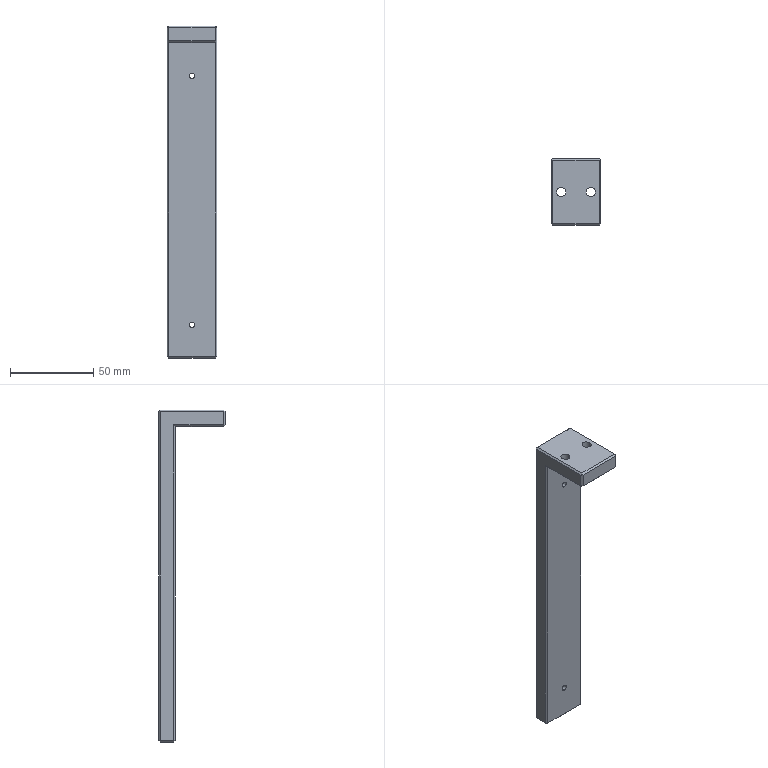Part | SolidWorks | features Chamfer 2, HoleWzd 2, Extrusion 1, ICE 1 | 1 solid | 47 faces | box 30 x 40 x 200 mm | volume 67180 mm3 | plane 35 | cylinder 12 | commonest cylinder face diameters 3.3 x4 5.5 x4 10 x4
STEP:
#1=CARTESIAN_POINT('',(15.,-5.,68.35));
#2=VERTEX_POINT('',#1);
#3=CARTESIAN_POINT('',(15.,-5.,71.65));
#4=VERTEX_POINT('',#3);
#5=CARTESIAN_POINT('',(15.,-5.,70.));
#6=DIRECTION('',(0.,1.,0.));
#7=DIRECTION('',(0.,0.,1.));
#8=AXIS2_PLACEMENT_3D('',#5,#6,#7);
#9=CIRCLE('',#8,1.65);
#10=EDGE_CURVE('',#2,#4,#9,.T.);
#11=ORIENTED_EDGE('',*,*,#10,.F.);
#12=CARTESIAN_POINT('',(15.,5.,68.35));
#13=VERTEX_POINT('',#12);
#14=CARTESIAN_POINT('',(15.,5.,68.35));
#15=DIRECTION('',(0.,1.,0.));
#16=VECTOR('',#15,1000.);
#17=LINE('',#14,#16);
#18=EDGE_CURVE('',#2,#13,#17,.T.);
#19=ORIENTED_EDGE('',*,*,#18,.T.);
#20=CARTESIAN_POINT('',(15.,5.,71.65));
#21=VERTEX_POINT('',#20);
#22=CARTESIAN_POINT('',(15.,5.,70.));
#23=DIRECTION('',(0.,1.,0.));
#24=DIRECTION('',(0.,0.,1.));
#25=AXIS2_PLACEMENT_3D('',#22,#23,#24);
#26=CIRCLE('',#25,1.65);
#27=EDGE_CURVE('',#13,#21,#26,.T.);
#28=ORIENTED_EDGE('',*,*,#27,.T.);
#29=CARTESIAN_POINT('',(15.,5.,71.65));
#30=DIRECTION('',(0.,1.,0.));
#31=VECTOR('',#30,1000.);
#32=LINE('',#29,#31);
#33=EDGE_CURVE('',#4,#21,#32,.T.);
#34=ORIENTED_EDGE('',*,*,#33,.F.);
#35=EDGE_LOOP('',(#11,#19,#28,#34));
#36=FACE_OUTER_BOUND('',#35,.T.);
#37=CARTESIAN_POINT('',(15.,5.,70.));
#38=DIRECTION('',(0.,1.,0.));
#39=DIRECTION('',(0.,0.,1.));
#40=AXIS2_PLACEMENT_3D('',#37,#38,#39);
#41=CYLINDRICAL_SURFACE('',#40,1.65);
#42=ADVANCED_FACE('',(#36),#41,.F.);
#43=CARTESIAN_POINT('',(15.,-5.,-81.65));
#44=VERTEX_POINT('',#43);
#45=CARTESIAN_POINT('',(15.,-5.,-78.35));
#46=VERTEX_POINT('',#45);
#47=CARTESIAN_POINT('',(15.,-5.,-80.));
#48=DIRECTION('',(0.,1.,0.));
#49=DIRECTION('',(0.,0.,1.));
#50=AXIS2_PLACEMENT_3D('',#47,#48,#49);
#51=CIRCLE('',#50,1.65);
#52=EDGE_CURVE('',#44,#46,#51,.T.);
#53=ORIENTED_EDGE('',*,*,#52,.F.);
#54=CARTESIAN_POINT('',(15.,5.,-81.65));
#55=VERTEX_POINT('',#54);
#56=CARTESIAN_POINT('',(15.,5.,-81.65));
#57=DIRECTION('',(0.,1.,0.));
#58=VECTOR('',#57,1000.);
#59=LINE('',#56,#58);
#60=EDGE_CURVE('',#44,#55,#59,.T.);
#61=ORIENTED_EDGE('',*,*,#60,.T.);
#62=CARTESIAN_POINT('',(15.,5.,-78.35));
#63=VERTEX_POINT('',#62);
#64=CARTESIAN_POINT('',(15.,5.,-80.));
#65=DIRECTION('',(0.,1.,0.));
#66=DIRECTION('',(0.,0.,1.));
#67=AXIS2_PLACEMENT_3D('',#64,#65,#66);
#68=CIRCLE('',#67,1.65);
#69=EDGE_CURVE('',#55,#63,#68,.T.);
#70=ORIENTED_EDGE('',*,*,#69,.T.);
#71=CARTESIAN_POINT('',(15.,5.,-78.35));
#72=DIRECTION('',(0.,1.,0.));
#73=VECTOR('',#72,1000.);
#74=LINE('',#71,#73);
#75=EDGE_CURVE('',#46,#63,#74,.T.);
#76=ORIENTED_EDGE('',*,*,#75,.F.);
#77=EDGE_LOOP('',(#53,#61,#70,#76));
#78=FACE_OUTER_BOUND('',#77,.T.);
#79=CARTESIAN_POINT('',(15.,5.,-80.));
#80=DIRECTION('',(0.,1.,0.));
#81=DIRECTION('',(0.,0.,1.));
#82=AXIS2_PLACEMENT_3D('',#79,#80,#81);
#83=CYLINDRICAL_SURFACE('',#82,1.65);
#84=ADVANCED_FACE('',(#78),#83,.F.);
#85=CARTESIAN_POINT('',(29.,-15.,95.7));
#86=VERTEX_POINT('',#85);
#87=CARTESIAN_POINT('',(19.,-15.,95.7));
#88=VERTEX_POINT('',#87);
#89=CARTESIAN_POINT('',(24.,-15.,95.7));
#90=DIRECTION('',(0.,0.,-1.));
#91=DIRECTION('',(-1.,0.,0.));
#92=AXIS2_PLACEMENT_3D('',#89,#90,#91);
#93=CIRCLE('',#92,5.);
#94=EDGE_CURVE('',#86,#88,#93,.T.);
#95=ORIENTED_EDGE('',*,*,#94,.F.);
#96=CARTESIAN_POINT('',(29.,-15.,90.));
#97=VERTEX_POINT('',#96);
#98=CARTESIAN_POINT('',(29.,-15.,90.));
#99=DIRECTION('',(0.,0.,-1.));
#100=VECTOR('',#99,1000.);
#101=LINE('',#98,#100);
#102=EDGE_CURVE('',#86,#97,#101,.T.);
#103=ORIENTED_EDGE('',*,*,#102,.T.);
#104=CARTESIAN_POINT('',(19.,-15.,90.));
#105=VERTEX_POINT('',#104);
#106=CARTESIAN_POINT('',(24.,-15.,90.));
#107=DIRECTION('',(0.,0.,-1.));
#108=DIRECTION('',(-1.,0.,0.));
#109=AXIS2_PLACEMENT_3D('',#106,#107,#108);
#110=CIRCLE('',#109,5.);
#111=EDGE_CURVE('',#97,#105,#110,.T.);
#112=ORIENTED_EDGE('',*,*,#111,.T.);
#113=CARTESIAN_POINT('',(19.,-15.,90.));
#114=DIRECTION('',(0.,0.,-1.));
#115=VECTOR('',#114,1000.);
#116=LINE('',#113,#115);
#117=EDGE_CURVE('',#88,#105,#116,.T.);
#118=ORIENTED_EDGE('',*,*,#117,.F.);
#119=EDGE_LOOP('',(#95,#103,#112,#118));
#120=FACE_OUTER_BOUND('',#119,.T.);
#121=CARTESIAN_POINT('',(24.,-15.,90.));
#122=DIRECTION('',(0.,0.,-1.));
#123=DIRECTION('',(-1.,0.,0.));
#124=AXIS2_PLACEMENT_3D('',#121,#122,#123);
#125=CYLINDRICAL_SURFACE('',#124,5.);
#126=ADVANCED_FACE('',(#120),#125,.F.);
#127=CARTESIAN_POINT('',(26.75,-15.,100.));
#128=VERTEX_POINT('',#127);
#129=CARTESIAN_POINT('',(21.25,-15.,100.));
#130=VERTEX_POINT('',#129);
#131=CARTESIAN_POINT('',(24.,-15.,100.));
#132=DIRECTION('',(0.,0.,-1.));
#133=DIRECTION('',(-1.,0.,0.));
#134=AXIS2_PLACEMENT_3D('',#131,#132,#133);
#135=CIRCLE('',#134,2.75);
#136=EDGE_CURVE('',#128,#130,#135,.T.);
#137=ORIENTED_EDGE('',*,*,#136,.F.);
#138=CARTESIAN_POINT('',(26.75,-15.,95.7));
#139=VERTEX_POINT('',#138);
#140=CARTESIAN_POINT('',(26.75,-15.,90.));
#141=DIRECTION('',(0.,0.,-1.));
#142=VECTOR('',#141,1000.);
#143=LINE('',#140,#142);
#144=EDGE_CURVE('',#128,#139,#143,.T.);
#145=ORIENTED_EDGE('',*,*,#144,.T.);
#146=CARTESIAN_POINT('',(21.25,-15.,95.7));
#147=VERTEX_POINT('',#146);
#148=CARTESIAN_POINT('',(24.,-15.,95.7));
#149=DIRECTION('',(0.,0.,-1.));
#150=DIRECTION('',(-1.,0.,0.));
#151=AXIS2_PLACEMENT_3D('',#148,#149,#150);
#152=CIRCLE('',#151,2.75);
#153=EDGE_CURVE('',#139,#147,#152,.T.);
#154=ORIENTED_EDGE('',*,*,#153,.T.);
#155=CARTESIAN_POINT('',(21.25,-15.,90.));
#156=DIRECTION('',(0.,0.,-1.));
#157=VECTOR('',#156,1000.);
#158=LINE('',#155,#157);
#159=EDGE_CURVE('',#130,#147,#158,.T.);
#160=ORIENTED_EDGE('',*,*,#159,.F.);
#161=EDGE_LOOP('',(#137,#145,#154,#160));
#162=FACE_OUTER_BOUND('',#161,.T.);
#163=CARTESIAN_POINT('',(24.,-15.,90.));
#164=DIRECTION('',(0.,0.,-1.));
#165=DIRECTION('',(-1.,0.,0.));
#166=AXIS2_PLACEMENT_3D('',#163,#164,#165);
#167=CYLINDRICAL_SURFACE('',#166,2.75);
#168=ADVANCED_FACE('',(#162),#167,.F.);
#169=CARTESIAN_POINT('',(11.,-15.,95.7));
#170=VERTEX_POINT('',#169);
#171=CARTESIAN_POINT('',(1.,-15.,95.7));
#172=VERTEX_POINT('',#171);
#173=CARTESIAN_POINT('',(6.,-15.,95.7));
#174=DIRECTION('',(0.,0.,-1.));
#175=DIRECTION('',(-1.,0.,0.));
#176=AXIS2_PLACEMENT_3D('',#173,#174,#175);
#177=CIRCLE('',#176,5.);
#178=EDGE_CURVE('',#170,#172,#177,.T.);
#179=ORIENTED_EDGE('',*,*,#178,.F.);
#180=CARTESIAN_POINT('',(11.,-15.,90.));
#181=VERTEX_POINT('',#180);
#182=CARTESIAN_POINT('',(11.,-15.,90.));
#183=DIRECTION('',(0.,0.,-1.));
#184=VECTOR('',#183,1000.);
#185=LINE('',#182,#184);
#186=EDGE_CURVE('',#170,#181,#185,.T.);
#187=ORIENTED_EDGE('',*,*,#186,.T.);
#188=CARTESIAN_POINT('',(1.,-15.,90.));
#189=VERTEX_POINT('',#188);
#190=CARTESIAN_POINT('',(6.,-15.,90.));
#191=DIRECTION('',(0.,0.,-1.));
#192=DIRECTION('',(-1.,0.,0.));
#193=AXIS2_PLACEMENT_3D('',#190,#191,#192);
#194=CIRCLE('',#193,5.);
#195=EDGE_CURVE('',#181,#189,#194,.T.);
#196=ORIENTED_EDGE('',*,*,#195,.T.);
#197=CARTESIAN_POINT('',(1.,-15.,90.));
#198=DIRECTION('',(0.,0.,-1.));
#199=VECTOR('',#198,1000.);
#200=LINE('',#197,#199);
#201=EDGE_CURVE('',#172,#189,#200,.T.);
#202=ORIENTED_EDGE('',*,*,#201,.F.);
#203=EDGE_LOOP('',(#179,#187,#196,#202));
#204=FACE_OUTER_BOUND('',#203,.T.);
#205=CARTESIAN_POINT('',(6.,-15.,90.));
#206=DIRECTION('',(0.,0.,-1.));
#207=DIRECTION('',(-1.,0.,0.));
#208=AXIS2_PLACEMENT_3D('',#205,#206,#207);
#209=CYLINDRICAL_SURFACE('',#208,5.);
#210=ADVANCED_FACE('',(#204),#209,.F.);
#211=CARTESIAN_POINT('',(8.75,-15.,100.));
#212=VERTEX_POINT('',#211);
#213=CARTESIAN_POINT('',(3.25,-15.,100.));
#214=VERTEX_POINT('',#213);
#215=CARTESIAN_POINT('',(6.,-15.,100.));
#216=DIRECTION('',(0.,0.,-1.));
#217=DIRECTION('',(-1.,0.,0.));
#218=AXIS2_PLACEMENT_3D('',#215,#216,#217);
#219=CIRCLE('',#218,2.75);
#220=EDGE_CURVE('',#212,#214,#219,.T.);
#221=ORIENTED_EDGE('',*,*,#220,.F.);
#222=CARTESIAN_POINT('',(8.75,-15.,95.7));
#223=VERTEX_POINT('',#222);
#224=CARTESIAN_POINT('',(8.75,-15.,90.));
#225=DIRECTION('',(0.,0.,-1.));
#226=VECTOR('',#225,1000.);
#227=LINE('',#224,#226);
#228=EDGE_CURVE('',#212,#223,#227,.T.);
#229=ORIENTED_EDGE('',*,*,#228,.T.);
#230=CARTESIAN_POINT('',(3.25,-15.,95.7));
#231=VERTEX_POINT('',#230);
#232=CARTESIAN_POINT('',(6.,-15.,95.7));
#233=DIRECTION('',(0.,0.,-1.));
#234=DIRECTION('',(-1.,0.,0.));
#235=AXIS2_PLACEMENT_3D('',#232,#233,#234);
#236=CIRCLE('',#235,2.75);
#237=EDGE_CURVE('',#223,#231,#236,.T.);
#238=ORIENTED_EDGE('',*,*,#237,.T.);
#239=CARTESIAN_POINT('',(3.25,-15.,90.));
#240=DIRECTION('',(0.,0.,-1.));
#241=VECTOR('',#240,1000.);
#242=LINE('',#239,#241);
#243=EDGE_CURVE('',#214,#231,#242,.T.);
#244=ORIENTED_EDGE('',*,*,#243,.F.);
#245=EDGE_LOOP('',(#221,#229,#238,#244));
#246=FACE_OUTER_BOUND('',#245,.T.);
#247=CARTESIAN_POINT('',(6.,-15.,90.));
#248=DIRECTION('',(0.,0.,-1.));
#249=DIRECTION('',(-1.,0.,0.));
#250=AXIS2_PLACEMENT_3D('',#247,#248,#249);
#251=CYLINDRICAL_SURFACE('',#250,2.75);
#252=ADVANCED_FACE('',(#246),#251,.F.);
#253=CARTESIAN_POINT('',(1.,4.,-100.));
#254=VERTEX_POINT('',#253);
#255=CARTESIAN_POINT('',(29.,4.,-100.));
#256=VERTEX_POINT('',#255);
#257=CARTESIAN_POINT('',(30.,4.,-100.));
#258=DIRECTION('',(1.,0.,0.));
#259=VECTOR('',#258,1000.);
#260=LINE('',#257,#259);
#261=EDGE_CURVE('',#254,#256,#260,.T.);
#262=ORIENTED_EDGE('',*,*,#261,.T.);
#263=CARTESIAN_POINT('',(29.,-4.,-100.));
#264=VERTEX_POINT('',#263);
#265=CARTESIAN_POINT('',(29.,-5.,-100.));
#266=DIRECTION('',(0.,-1.,0.));
#267=VECTOR('',#266,1000.);
#268=LINE('',#265,#267);
#269=EDGE_CURVE('',#256,#264,#268,.T.);
#270=ORIENTED_EDGE('',*,*,#269,.T.);
#271=CARTESIAN_POINT('',(1.,-4.,-100.));
#272=VERTEX_POINT('',#271);
#273=CARTESIAN_POINT('',(30.,-4.,-100.));
#274=DIRECTION('',(-1.,0.,0.));
#275=VECTOR('',#274,1000.);
#276=LINE('',#273,#275);
#277=EDGE_CURVE('',#264,#272,#276,.T.);
#278=ORIENTED_EDGE('',*,*,#277,.T.);
#279=CARTESIAN_POINT('',(1.,5.,-100.));
#280=DIRECTION('',(0.,1.,0.));
#281=VECTOR('',#280,1000.);
#282=LINE('',#279,#281);
#283=EDGE_CURVE('',#272,#254,#282,.T.);
#284=ORIENTED_EDGE('',*,*,#283,.T.);
#285=EDGE_LOOP('',(#262,#270,#278,#284));
#286=FACE_OUTER_BOUND('',#285,.T.);
#287=CARTESIAN_POINT('',(30.,5.,-100.));
#288=DIRECTION('',(0.,0.,1.));
#289=DIRECTION('',(1.,0.,0.));
#290=AXIS2_PLACEMENT_3D('',#287,#288,#289);
#291=PLANE('',#290);
#292=ADVANCED_FACE('',(#286),#291,.F.);
#293=CARTESIAN_POINT('',(15.,5.,70.));
#294=DIRECTION('',(0.,1.,0.));
#295=DIRECTION('',(0.,0.,1.));
#296=AXIS2_PLACEMENT_3D('',#293,#294,#295);
#297=CIRCLE('',#296,1.65);
#298=EDGE_CURVE('',#21,#13,#297,.T.);
#299=ORIENTED_EDGE('',*,*,#298,.F.);
#300=ORIENTED_EDGE('',*,*,#27,.F.);
#301=EDGE_LOOP('',(#299,#300));
#302=FACE_BOUND('',#301,.T.);
#303=CARTESIAN_POINT('',(15.,5.,-80.));
#304=DIRECTION('',(0.,1.,0.));
#305=DIRECTION('',(0.,0.,1.));
#306=AXIS2_PLACEMENT_3D('',#303,#304,#305);
#307=CIRCLE('',#306,1.65);
#308=EDGE_CURVE('',#63,#55,#307,.T.);
#309=ORIENTED_EDGE('',*,*,#308,.F.);
#310=ORIENTED_EDGE('',*,*,#69,.F.);
#311=EDGE_LOOP('',(#309,#310));
#312=FACE_BOUND('',#311,.T.);
#313=CARTESIAN_POINT('',(1.,5.,-99.));
#314=VERTEX_POINT('',#313);
#315=CARTESIAN_POINT('',(1.,5.,99.));
#316=VERTEX_POINT('',#315);
#317=CARTESIAN_POINT('',(1.,5.,100.));
#318=DIRECTION('',(0.,0.,1.));
#319=VECTOR('',#318,1000.);
#320=LINE('',#317,#319);
#321=EDGE_CURVE('',#314,#316,#320,.T.);
#322=ORIENTED_EDGE('',*,*,#321,.T.);
#323=CARTESIAN_POINT('',(29.,5.,99.));
#324=VERTEX_POINT('',#323);
#325=CARTESIAN_POINT('',(30.,5.,99.));
#326=DIRECTION('',(1.,0.,0.));
#327=VECTOR('',#326,1000.);
#328=LINE('',#325,#327);
#329=EDGE_CURVE('',#316,#324,#328,.T.);
#330=ORIENTED_EDGE('',*,*,#329,.T.);
#331=CARTESIAN_POINT('',(29.,5.,-99.));
#332=VERTEX_POINT('',#331);
#333=CARTESIAN_POINT('',(29.,5.,-100.));
#334=DIRECTION('',(0.,0.,-1.));
#335=VECTOR('',#334,1000.);
#336=LINE('',#333,#335);
#337=EDGE_CURVE('',#324,#332,#336,.T.);
#338=ORIENTED_EDGE('',*,*,#337,.T.);
#339=CARTESIAN_POINT('',(30.,5.,-99.));
#340=DIRECTION('',(-1.,0.,0.));
#341=VECTOR('',#340,1000.);
#342=LINE('',#339,#341);
#343=EDGE_CURVE('',#332,#314,#342,.T.);
#344=ORIENTED_EDGE('',*,*,#343,.T.);
#345=EDGE_LOOP('',(#322,#330,#338,#344));
#346=FACE_OUTER_BOUND('',#345,.T.);
#347=CARTESIAN_POINT('',(30.,5.,100.));
#348=DIRECTION('',(0.,-1.,0.));
#349=DIRECTION('',(0.,0.,-1.));
#350=AXIS2_PLACEMENT_3D('',#347,#348,#349);
#351=PLANE('',#350);
#352=ADVANCED_FACE('',(#302,#312,#346),#351,.F.);
#353=CARTESIAN_POINT('',(24.,-15.,100.));
#354=DIRECTION('',(0.,0.,-1.));
#355=DIRECTION('',(-1.,0.,0.));
#356=AXIS2_PLACEMENT_3D('',#353,#354,#355);
#357=CIRCLE('',#356,2.75);
#358=EDGE_CURVE('',#130,#128,#357,.T.);
#359=ORIENTED_EDGE('',*,*,#358,.T.);
#360=ORIENTED_EDGE('',*,*,#136,.T.);
#361=EDGE_LOOP('',(#359,#360));
#362=FACE_BOUND('',#361,.T.);
#363=CARTESIAN_POINT('',(6.,-15.,100.));
#364=DIRECTION('',(0.,0.,-1.));
#365=DIRECTION('',(-1.,0.,0.));
#366=AXIS2_PLACEMENT_3D('',#363,#364,#365);
#367=CIRCLE('',#366,2.75);
#368=EDGE_CURVE('',#214,#212,#367,.T.);
#369=ORIENTED_EDGE('',*,*,#368,.T.);
#370=ORIENTED_EDGE('',*,*,#220,.T.);
#371=EDGE_LOOP('',(#369,#370));
#372=FACE_BOUND('',#371,.T.);
#373=CARTESIAN_POINT('',(29.,-34.,100.));
#374=VERTEX_POINT('',#373);
#375=CARTESIAN_POINT('',(29.,4.,100.));
#376=VERTEX_POINT('',#375);
#377=CARTESIAN_POINT('',(29.,5.,100.));
#378=DIRECTION('',(0.,1.,0.));
#379=VECTOR('',#378,1000.);
#380=LINE('',#377,#379);
#381=EDGE_CURVE('',#374,#376,#380,.T.);
#382=ORIENTED_EDGE('',*,*,#381,.T.);
#383=CARTESIAN_POINT('',(1.,4.,100.));
#384=VERTEX_POINT('',#383);
#385=CARTESIAN_POINT('',(30.,4.,100.));
#386=DIRECTION('',(-1.,0.,0.));
#387=VECTOR('',#386,1000.);
#388=LINE('',#385,#387);
#389=EDGE_CURVE('',#376,#384,#388,.T.);
#390=ORIENTED_EDGE('',*,*,#389,.T.);
#391=CARTESIAN_POINT('',(1.,-34.,100.));
#392=VERTEX_POINT('',#391);
#393=CARTESIAN_POINT('',(1.,5.,100.));
#394=DIRECTION('',(0.,-1.,0.));
#395=VECTOR('',#394,1000.);
#396=LINE('',#393,#395);
#397=EDGE_CURVE('',#384,#392,#396,.T.);
#398=ORIENTED_EDGE('',*,*,#397,.T.);
#399=CARTESIAN_POINT('',(30.,-34.,100.));
#400=DIRECTION('',(1.,0.,0.));
#401=VECTOR('',#400,1000.);
#402=LINE('',#399,#401);
#403=EDGE_CURVE('',#392,#374,#402,.T.);
#404=ORIENTED_EDGE('',*,*,#403,.T.);
#405=EDGE_LOOP('',(#382,#390,#398,#404));
#406=FACE_OUTER_BOUND('',#405,.T.);
#407=CARTESIAN_POINT('',(30.,5.,100.));
#408=DIRECTION('',(0.,0.,-1.));
#409=DIRECTION('',(-1.,0.,0.));
#410=AXIS2_PLACEMENT_3D('',#407,#408,#409);
#411=PLANE('',#410);
#412=ADVANCED_FACE('',(#362,#372,#406),#411,.F.);
#413=CARTESIAN_POINT('',(15.,-5.,70.));
#414=DIRECTION('',(0.,1.,0.));
#415=DIRECTION('',(0.,0.,1.));
#416=AXIS2_PLACEMENT_3D('',#413,#414,#415);
#417=CIRCLE('',#416,1.65);
#418=EDGE_CURVE('',#4,#2,#417,.T.);
#419=ORIENTED_EDGE('',*,*,#418,.T.);
#420=ORIENTED_EDGE('',*,*,#10,.T.);
#421=EDGE_LOOP('',(#419,#420));
#422=FACE_BOUND('',#421,.T.);
#423=CARTESIAN_POINT('',(15.,-5.,-80.));
#424=DIRECTION('',(0.,1.,0.));
#425=DIRECTION('',(0.,0.,1.));
#426=AXIS2_PLACEMENT_3D('',#423,#424,#425);
#427=CIRCLE('',#426,1.65);
#428=EDGE_CURVE('',#46,#44,#427,.T.);
#429=ORIENTED_EDGE('',*,*,#428,.T.);
#430=ORIENTED_EDGE('',*,*,#52,.T.);
#431=EDGE_LOOP('',(#429,#430));
#432=FACE_BOUND('',#431,.T.);
#433=CARTESIAN_POINT('',(1.,-5.,-99.));
#434=VERTEX_POINT('',#433);
#435=CARTESIAN_POINT('',(29.,-5.,-99.));
#436=VERTEX_POINT('',#435);
#437=CARTESIAN_POINT('',(30.,-5.,-99.));
#438=DIRECTION('',(1.,0.,0.));
#439=VECTOR('',#438,1000.);
#440=LINE('',#437,#439);
#441=EDGE_CURVE('',#434,#436,#440,.T.);
#442=ORIENTED_EDGE('',*,*,#441,.T.);
#443=CARTESIAN_POINT('',(29.,-5.,90.));
#444=VERTEX_POINT('',#443);
#445=CARTESIAN_POINT('',(29.,-5.,90.));
#446=DIRECTION('',(0.,0.,1.));
#447=VECTOR('',#446,1000.);
#448=LINE('',#445,#447);
#449=EDGE_CURVE('',#436,#444,#448,.T.);
#450=ORIENTED_EDGE('',*,*,#449,.T.);
#451=CARTESIAN_POINT('',(1.,-5.,90.));
#452=VERTEX_POINT('',#451);
#453=CARTESIAN_POINT('',(0.,-5.,90.));
#454=DIRECTION('',(-1.,0.,0.));
#455=VECTOR('',#454,1000.);
#456=LINE('',#453,#455);
#457=EDGE_CURVE('',#444,#452,#456,.T.);
#458=ORIENTED_EDGE('',*,*,#457,.T.);
#459=CARTESIAN_POINT('',(1.,-5.,100.));
#460=DIRECTION('',(0.,0.,-1.));
#461=VECTOR('',#460,1000.);
#462=LINE('',#459,#461);
#463=EDGE_CURVE('',#452,#434,#462,.T.);
#464=ORIENTED_EDGE('',*,*,#463,.T.);
#465=EDGE_LOOP('',(#442,#450,#458,#464));
#466=FACE_OUTER_BOUND('',#465,.T.);
#467=CARTESIAN_POINT('',(30.,-5.,100.));
#468=DIRECTION('',(0.,1.,0.));
#469=DIRECTION('',(0.,0.,1.));
#470=AXIS2_PLACEMENT_3D('',#467,#468,#469);
#471=PLANE('',#470);
#472=ADVANCED_FACE('',(#422,#432,#466),#471,.F.);
#473=CARTESIAN_POINT('',(30.,-34.,91.));
#474=VERTEX_POINT('',#473);
#475=CARTESIAN_POINT('',(30.,-4.,91.));
#476=VERTEX_POINT('',#475);
#477=CARTESIAN_POINT('',(30.,-5.,91.));
#478=DIRECTION('',(0.,1.,0.));
#479=VECTOR('',#478,1000.);
#480=LINE('',#477,#479);
#481=EDGE_CURVE('',#474,#476,#480,.T.);
#482=ORIENTED_EDGE('',*,*,#481,.T.);
#483=CARTESIAN_POINT('',(30.,-4.,-99.));
#484=VERTEX_POINT('',#483);
#485=CARTESIAN_POINT('',(30.,-4.,-100.));
#486=DIRECTION('',(0.,0.,-1.));
#487=VECTOR('',#486,1000.);
#488=LINE('',#485,#487);
#489=EDGE_CURVE('',#476,#484,#488,.T.);
#490=ORIENTED_EDGE('',*,*,#489,.T.);
#491=CARTESIAN_POINT('',(30.,4.,-99.));
#492=VERTEX_POINT('',#491);
#493=CARTESIAN_POINT('',(30.,5.,-99.));
#494=DIRECTION('',(0.,1.,0.));
#495=VECTOR('',#494,1000.);
#496=LINE('',#493,#495);
#497=EDGE_CURVE('',#484,#492,#496,.T.);
#498=ORIENTED_EDGE('',*,*,#497,.T.);
#499=CARTESIAN_POINT('',(30.,4.,99.));
#500=VERTEX_POINT('',#499);
#501=CARTESIAN_POINT('',(30.,4.,100.));
#502=DIRECTION('',(0.,0.,1.));
#503=VECTOR('',#502,1000.);
#504=LINE('',#501,#503);
#505=EDGE_CURVE('',#492,#500,#504,.T.);
#506=ORIENTED_EDGE('',*,*,#505,.T.);
#507=CARTESIAN_POINT('',(30.,-34.,99.));
#508=VERTEX_POINT('',#507);
#509=CARTESIAN_POINT('',(30.,-35.,99.));
#510=DIRECTION('',(0.,-1.,0.));
#511=VECTOR('',#510,1000.);
#512=LINE('',#509,#511);
#513=EDGE_CURVE('',#500,#508,#512,.T.);
#514=ORIENTED_EDGE('',*,*,#513,.T.);
#515=CARTESIAN_POINT('',(30.,-34.,0.));
#516=DIRECTION('',(0.,0.,-1.));
#517=VECTOR('',#516,1000.);
#518=LINE('',#515,#517);
#519=EDGE_CURVE('',#508,#474,#518,.T.);
#520=ORIENTED_EDGE('',*,*,#519,.T.);
#521=EDGE_LOOP('',(#482,#490,#498,#506,#514,#520));
#522=FACE_OUTER_BOUND('',#521,.T.);
#523=CARTESIAN_POINT('',(30.,0.,0.));
#524=DIRECTION('',(1.,0.,0.));
#525=DIRECTION('',(0.,0.,-1.));
#526=AXIS2_PLACEMENT_3D('',#523,#524,#525);
#527=PLANE('',#526);
#528=ADVANCED_FACE('',(#522),#527,.T.);
#529=CARTESIAN_POINT('',(0.,-34.,99.));
#530=VERTEX_POINT('',#529);
#531=CARTESIAN_POINT('',(0.,4.,99.));
#532=VERTEX_POINT('',#531);
#533=CARTESIAN_POINT('',(0.,0.,99.));
#534=DIRECTION('',(0.,1.,0.));
#535=VECTOR('',#534,1000.);
#536=LINE('',#533,#535);
#537=EDGE_CURVE('',#530,#532,#536,.T.);
#538=ORIENTED_EDGE('',*,*,#537,.T.);
#539=CARTESIAN_POINT('',(0.,4.,-99.));
#540=VERTEX_POINT('',#539);
#541=CARTESIAN_POINT('',(0.,4.,0.));
#542=DIRECTION('',(0.,0.,-1.));
#543=VECTOR('',#542,1000.);
#544=LINE('',#541,#543);
#545=EDGE_CURVE('',#532,#540,#544,.T.);
#546=ORIENTED_EDGE('',*,*,#545,.T.);
#547=CARTESIAN_POINT('',(0.,-4.,-99.));
#548=VERTEX_POINT('',#547);
#549=CARTESIAN_POINT('',(0.,0.,-99.));
#550=DIRECTION('',(0.,-1.,0.));
#551=VECTOR('',#550,1000.);
#552=LINE('',#549,#551);
#553=EDGE_CURVE('',#540,#548,#552,.T.);
#554=ORIENTED_EDGE('',*,*,#553,.T.);
#555=CARTESIAN_POINT('',(0.,-4.,91.));
#556=VERTEX_POINT('',#555);
#557=CARTESIAN_POINT('',(0.,-4.,0.));
#558=DIRECTION('',(0.,0.,1.));
#559=VECTOR('',#558,1000.);
#560=LINE('',#557,#559);
#561=EDGE_CURVE('',#548,#556,#560,.T.);
#562=ORIENTED_EDGE('',*,*,#561,.T.);
#563=CARTESIAN_POINT('',(0.,-34.,91.));
#564=VERTEX_POINT('',#563);
#565=CARTESIAN_POINT('',(0.,0.,91.));
#566=DIRECTION('',(0.,-1.,0.));
#567=VECTOR('',#566,1000.);
#568=LINE('',#565,#567);
#569=EDGE_CURVE('',#556,#564,#568,.T.);
#570=ORIENTED_EDGE('',*,*,#569,.T.);
#571=CARTESIAN_POINT('',(0.,-34.,100.));
#572=DIRECTION('',(0.,0.,1.));
#573=VECTOR('',#572,1000.);
#574=LINE('',#571,#573);
#575=EDGE_CURVE('',#564,#530,#574,.T.);
#576=ORIENTED_EDGE('',*,*,#575,.T.);
#577=EDGE_LOOP('',(#538,#546,#554,#562,#570,#576));
#578=FACE_OUTER_BOUND('',#577,.T.);
#579=CARTESIAN_POINT('',(0.,0.,0.));
#580=DIRECTION('',(1.,0.,0.));
#581=DIRECTION('',(0.,0.,-1.));
#582=AXIS2_PLACEMENT_3D('',#579,#580,#581);
#583=PLANE('',#582);
#584=ADVANCED_FACE('',(#578),#583,.F.);
#585=CARTESIAN_POINT('',(1.,-35.,91.));
#586=VERTEX_POINT('',#585);
#587=CARTESIAN_POINT('',(29.,-35.,91.));
#588=VERTEX_POINT('',#587);
#589=CARTESIAN_POINT('',(30.,-35.,91.));
#590=DIRECTION('',(1.,0.,0.));
#591=VECTOR('',#590,1000.);
#592=LINE('',#589,#591);
#593=EDGE_CURVE('',#586,#588,#592,.T.);
#594=ORIENTED_EDGE('',*,*,#593,.T.);
#595=CARTESIAN_POINT('',(29.,-35.,99.));
#596=VERTEX_POINT('',#595);
#597=CARTESIAN_POINT('',(29.,-35.,90.));
#598=DIRECTION('',(0.,0.,1.));
#599=VECTOR('',#598,1000.);
#600=LINE('',#597,#599);
#601=EDGE_CURVE('',#588,#596,#600,.T.);
#602=ORIENTED_EDGE('',*,*,#601,.T.);
#603=CARTESIAN_POINT('',(1.,-35.,99.));
#604=VERTEX_POINT('',#603);
#605=CARTESIAN_POINT('',(0.,-35.,99.));
#606=DIRECTION('',(-1.,0.,0.));
#607=VECTOR('',#606,1000.);
#608=LINE('',#605,#607);
#609=EDGE_CURVE('',#596,#604,#608,.T.);
#610=ORIENTED_EDGE('',*,*,#609,.T.);
#611=CARTESIAN_POINT('',(1.,-35.,90.));
#612=DIRECTION('',(0.,0.,-1.));
#613=VECTOR('',#612,1000.);
#614=LINE('',#611,#613);
#615=EDGE_CURVE('',#604,#586,#614,.T.);
#616=ORIENTED_EDGE('',*,*,#615,.T.);
#617=EDGE_LOOP('',(#594,#602,#610,#616));
#618=FACE_OUTER_BOUND('',#617,.T.);
#619=CARTESIAN_POINT('',(0.,-35.,90.));
#620=DIRECTION('',(0.,-1.,0.));
#621=DIRECTION('',(0.,0.,-1.));
#622=AXIS2_PLACEMENT_3D('',#619,#620,#621);
#623=PLANE('',#622);
#624=ADVANCED_FACE('',(#618),#623,.T.);
#625=CARTESIAN_POINT('',(6.,-15.,90.));
#626=DIRECTION('',(0.,0.,-1.));
#627=DIRECTION('',(-1.,0.,0.));
#628=AXIS2_PLACEMENT_3D('',#625,#626,#627);
#629=CIRCLE('',#628,5.);
#630=EDGE_CURVE('',#189,#181,#629,.T.);
#631=ORIENTED_EDGE('',*,*,#630,.F.);
#632=CARTESIAN_POINT('',(1.,0.,90.));
#633=DIRECTION('',(0.,1.,0.));
#634=VECTOR('',#633,1000.);
#635=LINE('',#632,#634);
#636=EDGE_CURVE('',#189,#452,#635,.T.);
#637=ORIENTED_EDGE('',*,*,#636,.T.);
#638=ORIENTED_EDGE('',*,*,#457,.F.);
#639=CARTESIAN_POINT('',(29.,-35.,90.));
#640=DIRECTION('',(0.,-1.,0.));
#641=VECTOR('',#640,1000.);
#642=LINE('',#639,#641);
#643=EDGE_CURVE('',#444,#97,#642,.T.);
#644=ORIENTED_EDGE('',*,*,#643,.T.);
#645=CARTESIAN_POINT('',(24.,-15.,90.));
#646=DIRECTION('',(0.,0.,-1.));
#647=DIRECTION('',(-1.,0.,0.));
#648=AXIS2_PLACEMENT_3D('',#645,#646,#647);
#649=CIRCLE('',#648,5.);
#650=EDGE_CURVE('',#105,#97,#649,.T.);
#651=ORIENTED_EDGE('',*,*,#650,.F.);
#652=ORIENTED_EDGE('',*,*,#111,.F.);
#653=CARTESIAN_POINT('',(29.,-34.,90.));
#654=VERTEX_POINT('',#653);
#655=CARTESIAN_POINT('',(29.,-35.,90.));
#656=DIRECTION('',(0.,-1.,0.));
#657=VECTOR('',#656,1000.);
#658=LINE('',#655,#657);
#659=EDGE_CURVE('',#97,#654,#658,.T.);
#660=ORIENTED_EDGE('',*,*,#659,.T.);
#661=CARTESIAN_POINT('',(1.,-34.,90.));
#662=VERTEX_POINT('',#661);
#663=CARTESIAN_POINT('',(0.,-34.,90.));
#664=DIRECTION('',(-1.,0.,0.));
#665=VECTOR('',#664,1000.);
#666=LINE('',#663,#665);
#667=EDGE_CURVE('',#654,#662,#666,.T.);
#668=ORIENTED_EDGE('',*,*,#667,.T.);
#669=CARTESIAN_POINT('',(1.,0.,90.));
#670=DIRECTION('',(0.,1.,0.));
#671=VECTOR('',#670,1000.);
#672=LINE('',#669,#671);
#673=EDGE_CURVE('',#662,#189,#672,.T.);
#674=ORIENTED_EDGE('',*,*,#673,.T.);
#675=ORIENTED_EDGE('',*,*,#195,.F.);
#676=EDGE_LOOP('',(#631,#637,#638,#644,#651,#652,#660,#668,#674,#675));
#677=FACE_OUTER_BOUND('',#676,.T.);
#678=CARTESIAN_POINT('',(0.,0.,90.));
#679=DIRECTION('',(0.,0.,1.));
#680=DIRECTION('',(1.,0.,0.));
#681=AXIS2_PLACEMENT_3D('',#678,#679,#680);
#682=PLANE('',#681);
#683=ADVANCED_FACE('',(#677),#682,.F.);
#684=ORIENTED_EDGE('',*,*,#228,.F.);
#685=ORIENTED_EDGE('',*,*,#368,.F.);
#686=ORIENTED_EDGE('',*,*,#243,.T.);
#687=CARTESIAN_POINT('',(6.,-15.,95.7));
#688=DIRECTION('',(0.,0.,-1.));
#689=DIRECTION('',(-1.,0.,0.));
#690=AXIS2_PLACEMENT_3D('',#687,#688,#689);
#691=CIRCLE('',#690,2.75);
#692=EDGE_CURVE('',#231,#223,#691,.T.);
#693=ORIENTED_EDGE('',*,*,#692,.T.);
#694=EDGE_LOOP('',(#684,#685,#686,#693));
#695=FACE_OUTER_BOUND('',#694,.T.);
#696=CARTESIAN_POINT('',(6.,-15.,90.));
#697=DIRECTION('',(0.,0.,-1.));
#698=DIRECTION('',(-1.,0.,0.));
#699=AXIS2_PLACEMENT_3D('',#696,#697,#698);
#700=CYLINDRICAL_SURFACE('',#699,2.75);
#701=ADVANCED_FACE('',(#695),#700,.F.);
#702=ORIENTED_EDGE('',*,*,#692,.F.);
#703=ORIENTED_EDGE('',*,*,#237,.F.);
#704=EDGE_LOOP('',(#702,#703));
#705=FACE_BOUND('',#704,.T.);
#706=CARTESIAN_POINT('',(6.,-15.,95.7));
#707=DIRECTION('',(0.,0.,-1.));
#708=DIRECTION('',(-1.,0.,0.));
#709=AXIS2_PLACEMENT_3D('',#706,#707,#708);
#710=CIRCLE('',#709,5.);
#711=EDGE_CURVE('',#172,#170,#710,.T.);
#712=ORIENTED_EDGE('',*,*,#711,.T.);
#713=ORIENTED_EDGE('',*,*,#178,.T.);
#714=EDGE_LOOP('',(#712,#713));
#715=FACE_OUTER_BOUND('',#714,.T.);
#716=CARTESIAN_POINT('',(8.75,-15.,95.7));
#717=DIRECTION('',(0.,0.,1.));
#718=DIRECTION('',(1.,0.,0.));
#719=AXIS2_PLACEMENT_3D('',#716,#717,#718);
#720=PLANE('',#719);
#721=ADVANCED_FACE('',(#705,#715),#720,.F.);
#722=ORIENTED_EDGE('',*,*,#186,.F.);
#723=ORIENTED_EDGE('',*,*,#711,.F.);
#724=ORIENTED_EDGE('',*,*,#201,.T.);
#725=ORIENTED_EDGE('',*,*,#630,.T.);
#726=EDGE_LOOP('',(#722,#723,#724,#725));
#727=FACE_OUTER_BOUND('',#726,.T.);
#728=CARTESIAN_POINT('',(6.,-15.,90.));
#729=DIRECTION('',(0.,0.,-1.));
#730=DIRECTION('',(-1.,0.,0.));
#731=AXIS2_PLACEMENT_3D('',#728,#729,#730);
#732=CYLINDRICAL_SURFACE('',#731,5.);
#733=ADVANCED_FACE('',(#727),#732,.F.);
#734=ORIENTED_EDGE('',*,*,#144,.F.);
#735=ORIENTED_EDGE('',*,*,#358,.F.);
#736=ORIENTED_EDGE('',*,*,#159,.T.);
#737=CARTESIAN_POINT('',(24.,-15.,95.7));
#738=DIRECTION('',(0.,0.,-1.));
#739=DIRECTION('',(-1.,0.,0.));
#740=AXIS2_PLACEMENT_3D('',#737,#738,#739);
#741=CIRCLE('',#740,2.75);
#742=EDGE_CURVE('',#147,#139,#741,.T.);
#743=ORIENTED_EDGE('',*,*,#742,.T.);
#744=EDGE_LOOP('',(#734,#735,#736,#743));
#745=FACE_OUTER_BOUND('',#744,.T.);
#746=CARTESIAN_POINT('',(24.,-15.,90.));
#747=DIRECTION('',(0.,0.,-1.));
#748=DIRECTION('',(-1.,0.,0.));
#749=AXIS2_PLACEMENT_3D('',#746,#747,#748);
#750=CYLINDRICAL_SURFACE('',#749,2.75);
#751=ADVANCED_FACE('',(#745),#750,.F.);
#752=ORIENTED_EDGE('',*,*,#742,.F.);
#753=ORIENTED_EDGE('',*,*,#153,.F.);
#754=EDGE_LOOP('',(#752,#753));
#755=FACE_BOUND('',#754,.T.);
#756=CARTESIAN_POINT('',(24.,-15.,95.7));
#757=DIRECTION('',(0.,0.,-1.));
#758=DIRECTION('',(-1.,0.,0.));
#759=AXIS2_PLACEMENT_3D('',#756,#757,#758);
#760=CIRCLE('',#759,5.);
#761=EDGE_CURVE('',#88,#86,#760,.T.);
#762=ORIENTED_EDGE('',*,*,#761,.T.);
#763=ORIENTED_EDGE('',*,*,#94,.T.);
#764=EDGE_LOOP('',(#762,#763));
#765=FACE_OUTER_BOUND('',#764,.T.);
#766=CARTESIAN_POINT('',(26.75,-15.,95.7));
#767=DIRECTION('',(0.,0.,1.));
#768=DIRECTION('',(1.,0.,0.));
#769=AXIS2_PLACEMENT_3D('',#766,#767,#768);
#770=PLANE('',#769);
#771=ADVANCED_FACE('',(#755,#765),#770,.F.);
#772=ORIENTED_EDGE('',*,*,#102,.F.);
#773=ORIENTED_EDGE('',*,*,#761,.F.);
#774=ORIENTED_EDGE('',*,*,#117,.T.);
#775=ORIENTED_EDGE('',*,*,#650,.T.);
#776=EDGE_LOOP('',(#772,#773,#774,#775));
#777=FACE_OUTER_BOUND('',#776,.T.);
#778=CARTESIAN_POINT('',(24.,-15.,90.));
#779=DIRECTION('',(0.,0.,-1.));
#780=DIRECTION('',(-1.,0.,0.));
#781=AXIS2_PLACEMENT_3D('',#778,#779,#780);
#782=CYLINDRICAL_SURFACE('',#781,5.);
#783=ADVANCED_FACE('',(#777),#782,.F.);
#784=CARTESIAN_POINT('',(29.,-34.5,99.5));
#785=DIRECTION('',(0.,-0.7071,-0.7071));
#786=VECTOR('',#785,1000.);
#787=LINE('',#784,#786);
#788=EDGE_CURVE('',#374,#596,#787,.T.);
#789=ORIENTED_EDGE('',*,*,#788,.F.);
#790=ORIENTED_EDGE('',*,*,#403,.F.);
#791=CARTESIAN_POINT('',(1.,-34.,100.));
#792=DIRECTION('',(0.,0.7071,0.7071));
#793=VECTOR('',#792,1000.);
#794=LINE('',#791,#793);
#795=EDGE_CURVE('',#604,#392,#794,.T.);
#796=ORIENTED_EDGE('',*,*,#795,.F.);
#797=ORIENTED_EDGE('',*,*,#609,.F.);
#798=EDGE_LOOP('',(#789,#790,#796,#797));
#799=FACE_OUTER_BOUND('',#798,.T.);
#800=CARTESIAN_POINT('',(30.,-34.,100.));
#801=DIRECTION('',(0.,-0.7071,0.7071));
#802=DIRECTION('',(-1.,0.,0.));
#803=AXIS2_PLACEMENT_3D('',#800,#801,#802);
#804=PLANE('',#803);
#805=ADVANCED_FACE('',(#799),#804,.T.);
#806=CARTESIAN_POINT('',(30.,-34.,99.));
#807=DIRECTION('',(0.7071,0.,-0.7071));
#808=VECTOR('',#807,1000.);
#809=LINE('',#806,#808);
#810=EDGE_CURVE('',#374,#508,#809,.T.);
#811=ORIENTED_EDGE('',*,*,#810,.F.);
#812=ORIENTED_EDGE('',*,*,#788,.T.);
#813=CARTESIAN_POINT('',(30.,-34.,99.));
#814=DIRECTION('',(-0.7071,-0.7071,0.));
#815=VECTOR('',#814,1000.);
#816=LINE('',#813,#815);
#817=EDGE_CURVE('',#508,#596,#816,.T.);
#818=ORIENTED_EDGE('',*,*,#817,.F.);
#819=EDGE_LOOP('',(#811,#812,#818));
#820=FACE_OUTER_BOUND('',#819,.T.);
#821=CARTESIAN_POINT('',(30.,-34.,99.));
#822=DIRECTION('',(0.5774,-0.5774,0.5774));
#823=DIRECTION('',(0.7071,0.7071,0.));
#824=AXIS2_PLACEMENT_3D('',#821,#822,#823);
#825=PLANE('',#824);
#826=ADVANCED_FACE('',(#820),#825,.T.);
#827=CARTESIAN_POINT('',(0.5,-34.5,99.));
#828=DIRECTION('',(-0.7071,0.7071,0.));
#829=VECTOR('',#828,1000.);
#830=LINE('',#827,#829);
#831=EDGE_CURVE('',#604,#530,#830,.T.);
#832=ORIENTED_EDGE('',*,*,#831,.F.);
#833=ORIENTED_EDGE('',*,*,#795,.T.);
#834=CARTESIAN_POINT('',(1.,-34.,100.));
#835=DIRECTION('',(0.7071,0.,0.7071));
#836=VECTOR('',#835,1000.);
#837=LINE('',#834,#836);
#838=EDGE_CURVE('',#530,#392,#837,.T.);
#839=ORIENTED_EDGE('',*,*,#838,.F.);
#840=EDGE_LOOP('',(#832,#833,#839));
#841=FACE_OUTER_BOUND('',#840,.T.);
#842=CARTESIAN_POINT('',(1.,-34.,100.));
#843=DIRECTION('',(-0.5774,-0.5774,0.5774));
#844=DIRECTION('',(0.7071,-0.7071,0.));
#845=AXIS2_PLACEMENT_3D('',#842,#843,#844);
#846=PLANE('',#845);
#847=ADVANCED_FACE('',(#841),#846,.T.);
#848=ORIENTED_EDGE('',*,*,#817,.T.);
#849=ORIENTED_EDGE('',*,*,#601,.F.);
#850=CARTESIAN_POINT('',(29.5,-34.5,91.));
#851=DIRECTION('',(-0.7071,-0.7071,0.));
#852=VECTOR('',#851,1000.);
#853=LINE('',#850,#852);
#854=EDGE_CURVE('',#474,#588,#853,.T.);
#855=ORIENTED_EDGE('',*,*,#854,.F.);
#856=ORIENTED_EDGE('',*,*,#519,.F.);
#857=EDGE_LOOP('',(#848,#849,#855,#856));
#858=FACE_OUTER_BOUND('',#857,.T.);
#859=CARTESIAN_POINT('',(29.,-35.,90.));
#860=DIRECTION('',(-0.7071,0.7071,0.));
#861=DIRECTION('',(0.,0.,1.));
#862=AXIS2_PLACEMENT_3D('',#859,#860,#861);
#863=PLANE('',#862);
#864=ADVANCED_FACE('',(#858),#863,.F.);
#865=CARTESIAN_POINT('',(29.5,4.5,99.5));
#866=VERTEX_POINT('',#865);
#867=CARTESIAN_POINT('',(31.333,2.667,97.667));
#868=DIRECTION('',(0.5774,-0.5774,-0.5774));
#869=VECTOR('',#868,1000.);
#870=LINE('',#867,#869);
#871=EDGE_CURVE('',#866,#500,#870,.T.);
#872=ORIENTED_EDGE('',*,*,#871,.F.);
#873=CARTESIAN_POINT('',(28.333,3.333,100.667));
#874=DIRECTION('',(-0.5774,-0.5774,0.5774));
#875=VECTOR('',#874,1000.);
#876=LINE('',#873,#875);
#877=EDGE_CURVE('',#866,#376,#876,.T.);
#878=ORIENTED_EDGE('',*,*,#877,.T.);
#879=ORIENTED_EDGE('',*,*,#381,.F.);
#880=ORIENTED_EDGE('',*,*,#810,.T.);
#881=ORIENTED_EDGE('',*,*,#513,.F.);
#882=EDGE_LOOP('',(#872,#878,#879,#880,#881));
#883=FACE_OUTER_BOUND('',#882,.T.);
#884=CARTESIAN_POINT('',(30.,0.,99.));
#885=DIRECTION('',(0.7071,0.,0.7071));
#886=DIRECTION('',(0.,1.,0.));
#887=AXIS2_PLACEMENT_3D('',#884,#885,#886);
#888=PLANE('',#887);
#889=ADVANCED_FACE('',(#883),#888,.T.);
#890=ORIENTED_EDGE('',*,*,#397,.F.);
#891=CARTESIAN_POINT('',(0.5,4.5,99.5));
#892=VERTEX_POINT('',#891);
#893=CARTESIAN_POINT('',(0.6667,4.333,99.667));
#894=DIRECTION('',(-0.5774,0.5774,-0.5774));
#895=VECTOR('',#894,1000.);
#896=LINE('',#893,#895);
#897=EDGE_CURVE('',#384,#892,#896,.T.);
#898=ORIENTED_EDGE('',*,*,#897,.T.);
#899=CARTESIAN_POINT('',(1.,5.,100.));
#900=DIRECTION('',(0.5774,0.5774,0.5774));
#901=VECTOR('',#900,1000.);
#902=LINE('',#899,#901);
#903=EDGE_CURVE('',#532,#892,#902,.T.);
#904=ORIENTED_EDGE('',*,*,#903,.F.);
#905=ORIENTED_EDGE('',*,*,#537,.F.);
#906=ORIENTED_EDGE('',*,*,#838,.T.);
#907=EDGE_LOOP('',(#890,#898,#904,#905,#906));
#908=FACE_OUTER_BOUND('',#907,.T.);
#909=CARTESIAN_POINT('',(1.,5.,100.));
#910=DIRECTION('',(0.7071,0.,-0.7071));
#911=DIRECTION('',(0.,-1.,0.));
#912=AXIS2_PLACEMENT_3D('',#909,#910,#911);
#913=PLANE('',#912);
#914=ADVANCED_FACE('',(#908),#913,.F.);
#915=ORIENTED_EDGE('',*,*,#831,.T.);
#916=ORIENTED_EDGE('',*,*,#575,.F.);
#917=CARTESIAN_POINT('',(0.,-34.,91.));
#918=DIRECTION('',(-0.7071,0.7071,0.));
#919=VECTOR('',#918,1000.);
#920=LINE('',#917,#919);
#921=EDGE_CURVE('',#586,#564,#920,.T.);
#922=ORIENTED_EDGE('',*,*,#921,.F.);
#923=ORIENTED_EDGE('',*,*,#615,.F.);
#924=EDGE_LOOP('',(#915,#916,#922,#923));
#925=FACE_OUTER_BOUND('',#924,.T.);
#926=CARTESIAN_POINT('',(0.,-34.,0.));
#927=DIRECTION('',(-0.7071,-0.7071,0.));
#928=DIRECTION('',(0.,0.,-1.));
#929=AXIS2_PLACEMENT_3D('',#926,#927,#928);
#930=PLANE('',#929);
#931=ADVANCED_FACE('',(#925),#930,.T.);
#932=CARTESIAN_POINT('',(29.,-34.,90.));
#933=DIRECTION('',(0.,0.7071,-0.7071));
#934=VECTOR('',#933,1000.);
#935=LINE('',#932,#934);
#936=EDGE_CURVE('',#588,#654,#935,.T.);
#937=ORIENTED_EDGE('',*,*,#936,.F.);
#938=ORIENTED_EDGE('',*,*,#593,.F.);
#939=CARTESIAN_POINT('',(1.,-34.5,90.5));
#940=DIRECTION('',(0.,-0.7071,0.7071));
#941=VECTOR('',#940,1000.);
#942=LINE('',#939,#941);
#943=EDGE_CURVE('',#662,#586,#942,.T.);
#944=ORIENTED_EDGE('',*,*,#943,.F.);
#945=ORIENTED_EDGE('',*,*,#667,.F.);
#946=EDGE_LOOP('',(#937,#938,#944,#945));
#947=FACE_OUTER_BOUND('',#946,.T.);
#948=CARTESIAN_POINT('',(0.,-35.,91.));
#949=DIRECTION('',(0.,-0.7071,-0.7071));
#950=DIRECTION('',(-1.,0.,0.));
#951=AXIS2_PLACEMENT_3D('',#948,#949,#950);
#952=PLANE('',#951);
#953=ADVANCED_FACE('',(#947),#952,.T.);
#954=ORIENTED_EDGE('',*,*,#854,.T.);
#955=ORIENTED_EDGE('',*,*,#936,.T.);
#956=CARTESIAN_POINT('',(29.,-34.,90.));
#957=DIRECTION('',(-0.7071,0.,-0.7071));
#958=VECTOR('',#957,1000.);
#959=LINE('',#956,#958);
#960=EDGE_CURVE('',#474,#654,#959,.T.);
#961=ORIENTED_EDGE('',*,*,#960,.F.);
#962=EDGE_LOOP('',(#954,#955,#961));
#963=FACE_OUTER_BOUND('',#962,.T.);
#964=CARTESIAN_POINT('',(29.,-34.,90.));
#965=DIRECTION('',(0.5774,-0.5774,-0.5774));
#966=DIRECTION('',(0.,0.7071,-0.7071));
#967=AXIS2_PLACEMENT_3D('',#964,#965,#966);
#968=PLANE('',#967);
#969=ADVANCED_FACE('',(#963),#968,.T.);
#970=ORIENTED_EDGE('',*,*,#337,.F.);
#971=CARTESIAN_POINT('',(-3.333,37.333,66.667));
#972=DIRECTION('',(0.5774,-0.5774,0.5774));
#973=VECTOR('',#972,1000.);
#974=LINE('',#971,#973);
#975=EDGE_CURVE('',#324,#866,#974,.T.);
#976=ORIENTED_EDGE('',*,*,#975,.T.);
#977=ORIENTED_EDGE('',*,*,#871,.T.);
#978=ORIENTED_EDGE('',*,*,#505,.F.);
#979=CARTESIAN_POINT('',(29.5,4.5,-99.));
#980=DIRECTION('',(0.7071,-0.7071,0.));
#981=VECTOR('',#980,1000.);
#982=LINE('',#979,#981);
#983=EDGE_CURVE('',#332,#492,#982,.T.);
#984=ORIENTED_EDGE('',*,*,#983,.F.);
#985=EDGE_LOOP('',(#970,#976,#977,#978,#984));
#986=FACE_OUTER_BOUND('',#985,.T.);
#987=CARTESIAN_POINT('',(30.,4.,0.));
#988=DIRECTION('',(0.7071,0.7071,0.));
#989=DIRECTION('',(0.,0.,-1.));
#990=AXIS2_PLACEMENT_3D('',#987,#988,#989);
#991=PLANE('',#990);
#992=ADVANCED_FACE('',(#986),#991,.T.);
#993=CARTESIAN_POINT('',(1.,5.,-99.));
#994=DIRECTION('',(0.,-0.7071,-0.7071));
#995=VECTOR('',#994,1000.);
#996=LINE('',#993,#995);
#997=EDGE_CURVE('',#314,#254,#996,.T.);
#998=ORIENTED_EDGE('',*,*,#997,.F.);
#999=ORIENTED_EDGE('',*,*,#343,.F.);
#1000=CARTESIAN_POINT('',(29.,4.,-100.));
#1001=DIRECTION('',(0.,0.7071,0.7071));
#1002=VECTOR('',#1001,1000.);
#1003=LINE('',#1000,#1002);
#1004=EDGE_CURVE('',#256,#332,#1003,.T.);
#1005=ORIENTED_EDGE('',*,*,#1004,.F.);
#1006=ORIENTED_EDGE('',*,*,#261,.F.);
#1007=EDGE_LOOP('',(#998,#999,#1005,#1006));
#1008=FACE_OUTER_BOUND('',#1007,.T.);
#1009=CARTESIAN_POINT('',(30.,5.,-99.));
#1010=DIRECTION('',(0.,-0.7071,0.7071));
#1011=DIRECTION('',(-1.,0.,0.));
#1012=AXIS2_PLACEMENT_3D('',#1009,#1010,#1011);
#1013=PLANE('',#1012);
#1014=ADVANCED_FACE('',(#1008),#1013,.F.);
#1015=ORIENTED_EDGE('',*,*,#903,.T.);
#1016=CARTESIAN_POINT('',(0.6667,4.667,99.333));
#1017=DIRECTION('',(0.5774,0.5774,-0.5774));
#1018=VECTOR('',#1017,1000.);
#1019=LINE('',#1016,#1018);
#1020=EDGE_CURVE('',#892,#316,#1019,.T.);
#1021=ORIENTED_EDGE('',*,*,#1020,.T.);
#1022=ORIENTED_EDGE('',*,*,#321,.F.);
#1023=CARTESIAN_POINT('',(1.,5.,-99.));
#1024=DIRECTION('',(0.7071,0.7071,0.));
#1025=VECTOR('',#1024,1000.);
#1026=LINE('',#1023,#1025);
#1027=EDGE_CURVE('',#540,#314,#1026,.T.);
#1028=ORIENTED_EDGE('',*,*,#1027,.F.);
#1029=ORIENTED_EDGE('',*,*,#545,.F.);
#1030=EDGE_LOOP('',(#1015,#1021,#1022,#1028,#1029));
#1031=FACE_OUTER_BOUND('',#1030,.T.);
#1032=CARTESIAN_POINT('',(1.,5.,100.));
#1033=DIRECTION('',(0.7071,-0.7071,0.));
#1034=DIRECTION('',(0.,0.,1.));
#1035=AXIS2_PLACEMENT_3D('',#1032,#1033,#1034);
#1036=PLANE('',#1035);
#1037=ADVANCED_FACE('',(#1031),#1036,.F.);
#1038=ORIENTED_EDGE('',*,*,#943,.T.);
#1039=ORIENTED_EDGE('',*,*,#921,.T.);
#1040=CARTESIAN_POINT('',(0.,-34.,91.));
#1041=DIRECTION('',(-0.7071,0.,0.7071));
#1042=VECTOR('',#1041,1000.);
#1043=LINE('',#1040,#1042);
#1044=EDGE_CURVE('',#662,#564,#1043,.T.);
#1045=ORIENTED_EDGE('',*,*,#1044,.F.);
#1046=EDGE_LOOP('',(#1038,#1039,#1045));
#1047=FACE_OUTER_BOUND('',#1046,.T.);
#1048=CARTESIAN_POINT('',(0.,-34.,91.));
#1049=DIRECTION('',(-0.5774,-0.5774,-0.5774));
#1050=DIRECTION('',(0.,0.7071,-0.7071));
#1051=AXIS2_PLACEMENT_3D('',#1048,#1049,#1050);
#1052=PLANE('',#1051);
#1053=ADVANCED_FACE('',(#1047),#1052,.T.);
#1054=ORIENTED_EDGE('',*,*,#659,.F.);
#1055=ORIENTED_EDGE('',*,*,#643,.F.);
#1056=CARTESIAN_POINT('',(-0.3333,-34.333,60.667));
#1057=DIRECTION('',(-0.5774,-0.5774,-0.5774));
#1058=VECTOR('',#1057,1000.);
#1059=LINE('',#1056,#1058);
#1060=EDGE_CURVE('',#476,#444,#1059,.T.);
#1061=ORIENTED_EDGE('',*,*,#1060,.F.);
#1062=ORIENTED_EDGE('',*,*,#481,.F.);
#1063=ORIENTED_EDGE('',*,*,#960,.T.);
#1064=EDGE_LOOP('',(#1054,#1055,#1061,#1062,#1063));
#1065=FACE_OUTER_BOUND('',#1064,.T.);
#1066=CARTESIAN_POINT('',(30.,0.,91.));
#1067=DIRECTION('',(0.7071,0.,-0.7071));
#1068=DIRECTION('',(0.,-1.,0.));
#1069=AXIS2_PLACEMENT_3D('',#1066,#1067,#1068);
#1070=PLANE('',#1069);
#1071=ADVANCED_FACE('',(#1065),#1070,.T.);
#1072=ORIENTED_EDGE('',*,*,#1004,.T.);
#1073=ORIENTED_EDGE('',*,*,#983,.T.);
#1074=CARTESIAN_POINT('',(29.,4.,-100.));
#1075=DIRECTION('',(0.7071,0.,0.7071));
#1076=VECTOR('',#1075,1000.);
#1077=LINE('',#1074,#1076);
#1078=EDGE_CURVE('',#256,#492,#1077,.T.);
#1079=ORIENTED_EDGE('',*,*,#1078,.F.);
#1080=EDGE_LOOP('',(#1072,#1073,#1079));
#1081=FACE_OUTER_BOUND('',#1080,.T.);
#1082=CARTESIAN_POINT('',(29.,4.,-100.));
#1083=DIRECTION('',(0.5774,0.5774,-0.5774));
#1084=DIRECTION('',(0.,0.7071,0.7071));
#1085=AXIS2_PLACEMENT_3D('',#1082,#1083,#1084);
#1086=PLANE('',#1085);
#1087=ADVANCED_FACE('',(#1081),#1086,.T.);
#1088=ORIENTED_EDGE('',*,*,#1027,.T.);
#1089=ORIENTED_EDGE('',*,*,#997,.T.);
#1090=CARTESIAN_POINT('',(0.5,4.,-99.5));
#1091=DIRECTION('',(0.7071,0.,-0.7071));
#1092=VECTOR('',#1091,1000.);
#1093=LINE('',#1090,#1092);
#1094=EDGE_CURVE('',#540,#254,#1093,.T.);
#1095=ORIENTED_EDGE('',*,*,#1094,.F.);
#1096=EDGE_LOOP('',(#1088,#1089,#1095));
#1097=FACE_OUTER_BOUND('',#1096,.T.);
#1098=CARTESIAN_POINT('',(1.,5.,-99.));
#1099=DIRECTION('',(-0.5774,0.5774,-0.5774));
#1100=DIRECTION('',(-0.7071,0.,0.7071));
#1101=AXIS2_PLACEMENT_3D('',#1098,#1099,#1100);
#1102=PLANE('',#1101);
#1103=ADVANCED_FACE('',(#1097),#1102,.T.);
#1104=ORIENTED_EDGE('',*,*,#1044,.T.);
#1105=ORIENTED_EDGE('',*,*,#569,.F.);
#1106=CARTESIAN_POINT('',(-2.333,-1.667,93.333));
#1107=DIRECTION('',(-0.5774,0.5774,0.5774));
#1108=VECTOR('',#1107,1000.);
#1109=LINE('',#1106,#1108);
#1110=EDGE_CURVE('',#452,#556,#1109,.T.);
#1111=ORIENTED_EDGE('',*,*,#1110,.F.);
#1112=ORIENTED_EDGE('',*,*,#636,.F.);
#1113=ORIENTED_EDGE('',*,*,#673,.F.);
#1114=EDGE_LOOP('',(#1104,#1105,#1111,#1112,#1113));
#1115=FACE_OUTER_BOUND('',#1114,.T.);
#1116=CARTESIAN_POINT('',(0.,0.,91.));
#1117=DIRECTION('',(0.7071,0.,0.7071));
#1118=DIRECTION('',(0.,-1.,0.));
#1119=AXIS2_PLACEMENT_3D('',#1116,#1117,#1118);
#1120=PLANE('',#1119);
#1121=ADVANCED_FACE('',(#1115),#1120,.F.);
#1122=ORIENTED_EDGE('',*,*,#1060,.T.);
#1123=ORIENTED_EDGE('',*,*,#449,.F.);
#1124=CARTESIAN_POINT('',(29.,-5.,-99.));
#1125=DIRECTION('',(-0.7071,-0.7071,0.));
#1126=VECTOR('',#1125,1000.);
#1127=LINE('',#1124,#1126);
#1128=EDGE_CURVE('',#484,#436,#1127,.T.);
#1129=ORIENTED_EDGE('',*,*,#1128,.F.);
#1130=ORIENTED_EDGE('',*,*,#489,.F.);
#1131=EDGE_LOOP('',(#1122,#1123,#1129,#1130));
#1132=FACE_OUTER_BOUND('',#1131,.T.);
#1133=CARTESIAN_POINT('',(30.,-4.,0.));
#1134=DIRECTION('',(0.7071,-0.7071,0.));
#1135=DIRECTION('',(0.,0.,1.));
#1136=AXIS2_PLACEMENT_3D('',#1133,#1134,#1135);
#1137=PLANE('',#1136);
#1138=ADVANCED_FACE('',(#1132),#1137,.T.);
#1139=ORIENTED_EDGE('',*,*,#1078,.T.);
#1140=ORIENTED_EDGE('',*,*,#497,.F.);
#1141=CARTESIAN_POINT('',(29.5,-4.,-99.5));
#1142=DIRECTION('',(0.7071,0.,0.7071));
#1143=VECTOR('',#1142,1000.);
#1144=LINE('',#1141,#1143);
#1145=EDGE_CURVE('',#264,#484,#1144,.T.);
#1146=ORIENTED_EDGE('',*,*,#1145,.F.);
#1147=ORIENTED_EDGE('',*,*,#269,.F.);
#1148=EDGE_LOOP('',(#1139,#1140,#1146,#1147));
#1149=FACE_OUTER_BOUND('',#1148,.T.);
#1150=CARTESIAN_POINT('',(30.,0.,-99.));
#1151=DIRECTION('',(0.7071,0.,-0.7071));
#1152=DIRECTION('',(0.,-1.,0.));
#1153=AXIS2_PLACEMENT_3D('',#1150,#1151,#1152);
#1154=PLANE('',#1153);
#1155=ADVANCED_FACE('',(#1149),#1154,.T.);
#1156=ORIENTED_EDGE('',*,*,#1094,.T.);
#1157=ORIENTED_EDGE('',*,*,#283,.F.);
#1158=CARTESIAN_POINT('',(1.,-4.,-100.));
#1159=DIRECTION('',(0.7071,0.,-0.7071));
#1160=VECTOR('',#1159,1000.);
#1161=LINE('',#1158,#1160);
#1162=EDGE_CURVE('',#548,#272,#1161,.T.);
#1163=ORIENTED_EDGE('',*,*,#1162,.F.);
#1164=ORIENTED_EDGE('',*,*,#553,.F.);
#1165=EDGE_LOOP('',(#1156,#1157,#1163,#1164));
#1166=FACE_OUTER_BOUND('',#1165,.T.);
#1167=CARTESIAN_POINT('',(1.,5.,-100.));
#1168=DIRECTION('',(0.7071,0.,0.7071));
#1169=DIRECTION('',(0.,1.,0.));
#1170=AXIS2_PLACEMENT_3D('',#1167,#1168,#1169);
#1171=PLANE('',#1170);
#1172=ADVANCED_FACE('',(#1166),#1171,.F.);
#1173=ORIENTED_EDGE('',*,*,#1110,.T.);
#1174=ORIENTED_EDGE('',*,*,#561,.F.);
#1175=CARTESIAN_POINT('',(0.5,-4.5,-99.));
#1176=DIRECTION('',(-0.7071,0.7071,0.));
#1177=VECTOR('',#1176,1000.);
#1178=LINE('',#1175,#1177);
#1179=EDGE_CURVE('',#434,#548,#1178,.T.);
#1180=ORIENTED_EDGE('',*,*,#1179,.F.);
#1181=ORIENTED_EDGE('',*,*,#463,.F.);
#1182=EDGE_LOOP('',(#1173,#1174,#1180,#1181));
#1183=FACE_OUTER_BOUND('',#1182,.T.);
#1184=CARTESIAN_POINT('',(1.,-5.,100.));
#1185=DIRECTION('',(0.7071,0.7071,0.));
#1186=DIRECTION('',(0.,0.,-1.));
#1187=AXIS2_PLACEMENT_3D('',#1184,#1185,#1186);
#1188=PLANE('',#1187);
#1189=ADVANCED_FACE('',(#1183),#1188,.F.);
#1190=ORIENTED_EDGE('',*,*,#1145,.T.);
#1191=ORIENTED_EDGE('',*,*,#1128,.T.);
#1192=CARTESIAN_POINT('',(29.,-5.,-99.));
#1193=DIRECTION('',(0.,-0.7071,0.7071));
#1194=VECTOR('',#1193,1000.);
#1195=LINE('',#1192,#1194);
#1196=EDGE_CURVE('',#264,#436,#1195,.T.);
#1197=ORIENTED_EDGE('',*,*,#1196,.F.);
#1198=EDGE_LOOP('',(#1190,#1191,#1197));
#1199=FACE_OUTER_BOUND('',#1198,.T.);
#1200=CARTESIAN_POINT('',(29.,-5.,-99.));
#1201=DIRECTION('',(0.5774,-0.5774,-0.5774));
#1202=DIRECTION('',(0.,0.7071,-0.7071));
#1203=AXIS2_PLACEMENT_3D('',#1200,#1201,#1202);
#1204=PLANE('',#1203);
#1205=ADVANCED_FACE('',(#1199),#1204,.T.);
#1206=ORIENTED_EDGE('',*,*,#1179,.T.);
#1207=ORIENTED_EDGE('',*,*,#1162,.T.);
#1208=CARTESIAN_POINT('',(1.,-4.,-100.));
#1209=DIRECTION('',(0.,0.7071,-0.7071));
#1210=VECTOR('',#1209,1000.);
#1211=LINE('',#1208,#1210);
#1212=EDGE_CURVE('',#434,#272,#1211,.T.);
#1213=ORIENTED_EDGE('',*,*,#1212,.F.);
#1214=EDGE_LOOP('',(#1206,#1207,#1213));
#1215=FACE_OUTER_BOUND('',#1214,.T.);
#1216=CARTESIAN_POINT('',(1.,-4.,-100.));
#1217=DIRECTION('',(-0.5774,-0.5774,-0.5774));
#1218=DIRECTION('',(0.7071,-0.7071,0.));
#1219=AXIS2_PLACEMENT_3D('',#1216,#1217,#1218);
#1220=PLANE('',#1219);
#1221=ADVANCED_FACE('',(#1215),#1220,.T.);
#1222=ORIENTED_EDGE('',*,*,#1196,.T.);
#1223=ORIENTED_EDGE('',*,*,#441,.F.);
#1224=ORIENTED_EDGE('',*,*,#1212,.T.);
#1225=ORIENTED_EDGE('',*,*,#277,.F.);
#1226=EDGE_LOOP('',(#1222,#1223,#1224,#1225));
#1227=FACE_OUTER_BOUND('',#1226,.T.);
#1228=CARTESIAN_POINT('',(30.,-4.,-100.));
#1229=DIRECTION('',(0.,0.7071,0.7071));
#1230=DIRECTION('',(-1.,0.,0.));
#1231=AXIS2_PLACEMENT_3D('',#1228,#1229,#1230);
#1232=PLANE('',#1231);
#1233=ADVANCED_FACE('',(#1227),#1232,.F.);
#1234=ORIENTED_EDGE('',*,*,#975,.F.);
#1235=ORIENTED_EDGE('',*,*,#329,.F.);
#1236=ORIENTED_EDGE('',*,*,#1020,.F.);
#1237=ORIENTED_EDGE('',*,*,#897,.F.);
#1238=ORIENTED_EDGE('',*,*,#389,.F.);
#1239=ORIENTED_EDGE('',*,*,#877,.F.);
#1240=EDGE_LOOP('',(#1234,#1235,#1236,#1237,#1238,#1239));
#1241=FACE_OUTER_BOUND('',#1240,.T.);
#1242=CARTESIAN_POINT('',(30.,4.,100.));
#1243=DIRECTION('',(0.,-0.7071,-0.7071));
#1244=DIRECTION('',(-1.,0.,0.));
#1245=AXIS2_PLACEMENT_3D('',#1242,#1243,#1244);
#1246=PLANE('',#1245);
#1247=ADVANCED_FACE('',(#1241),#1246,.F.);
#1248=ORIENTED_EDGE('',*,*,#60,.F.);
#1249=ORIENTED_EDGE('',*,*,#428,.F.);
#1250=ORIENTED_EDGE('',*,*,#75,.T.);
#1251=ORIENTED_EDGE('',*,*,#308,.T.);
#1252=EDGE_LOOP('',(#1248,#1249,#1250,#1251));
#1253=FACE_OUTER_BOUND('',#1252,.T.);
#1254=CARTESIAN_POINT('',(15.,5.,-80.));
#1255=DIRECTION('',(0.,1.,0.));
#1256=DIRECTION('',(0.,0.,1.));
#1257=AXIS2_PLACEMENT_3D('',#1254,#1255,#1256);
#1258=CYLINDRICAL_SURFACE('',#1257,1.65);
#1259=ADVANCED_FACE('',(#1253),#1258,.F.);
#1260=ORIENTED_EDGE('',*,*,#18,.F.);
#1261=ORIENTED_EDGE('',*,*,#418,.F.);
#1262=ORIENTED_EDGE('',*,*,#33,.T.);
#1263=ORIENTED_EDGE('',*,*,#298,.T.);
#1264=EDGE_LOOP('',(#1260,#1261,#1262,#1263));
#1265=FACE_OUTER_BOUND('',#1264,.T.);
#1266=CARTESIAN_POINT('',(15.,5.,70.));
#1267=DIRECTION('',(0.,1.,0.));
#1268=DIRECTION('',(0.,0.,1.));
#1269=AXIS2_PLACEMENT_3D('',#1266,#1267,#1268);
#1270=CYLINDRICAL_SURFACE('',#1269,1.65);
#1271=ADVANCED_FACE('',(#1265),#1270,.F.);
#1272=CLOSED_SHELL('',(#42,#84,#126,#168,#210,#252,#292,#352,#412,#472,#528,#584,#624,#683,#701,#721,#733,#751,#771,#783,#805,#826,#847,#864,#889,#914,#931,#953,#969,#992,#1014,#1037,#1053,#1071,#1087,#1103,#1121,#1138,#1155,#1172,#1189,#1205,#1221,#1233,#1247,#1259,#1271));
#1273=MANIFOLD_SOLID_BREP('',#1272);
#1274=CARTESIAN_POINT('',(0.,0.,0.));
#1275=DIRECTION('',(0.,0.,1.));
#1276=DIRECTION('',(1.,0.,0.));
#1277=AXIS2_PLACEMENT_3D('',#1274,#1275,#1276);
#1278=(LENGTH_UNIT()NAMED_UNIT(*)SI_UNIT(.MILLI.,.METRE.));
#1279=UNCERTAINTY_MEASURE_WITH_UNIT(LENGTH_MEASURE(0.00001),#1278,'','');
#1280=(NAMED_UNIT(*)PLANE_ANGLE_UNIT()SI_UNIT($,.RADIAN.));
#1281=(NAMED_UNIT(*)SI_UNIT($,.STERADIAN.)SOLID_ANGLE_UNIT());
#1282=(GEOMETRIC_REPRESENTATION_CONTEXT(3)GLOBAL_UNCERTAINTY_ASSIGNED_CONTEXT((#1279))GLOBAL_UNIT_ASSIGNED_CONTEXT((#1278,#1280,#1281))REPRESENTATION_CONTEXT('',''));
#1283=ADVANCED_BREP_SHAPE_REPRESENTATION('',(#1273,#1277),#1282);